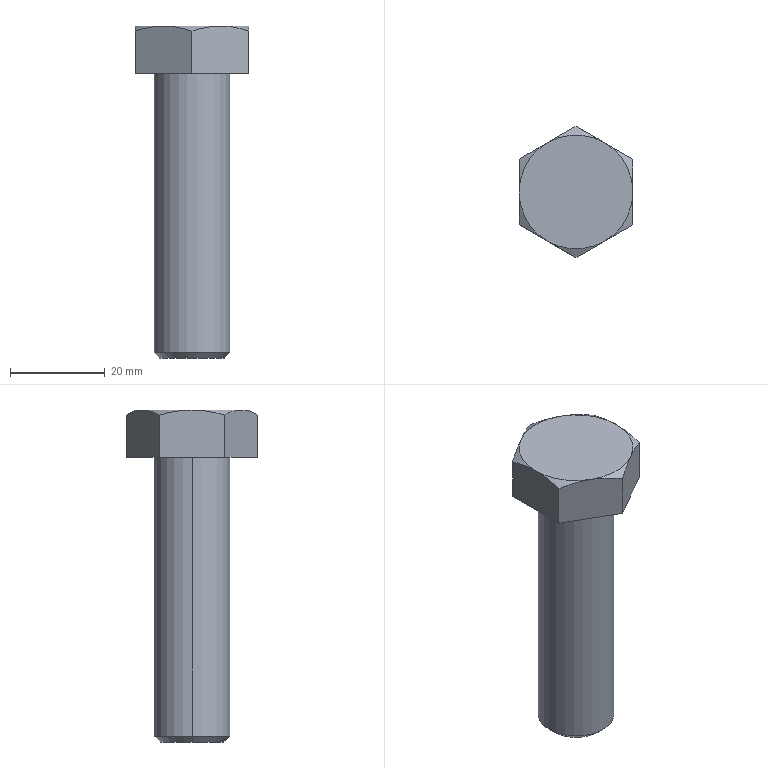Part | SolidWorks | features BaseBody 1 | 1 solid | 19 faces | box 24 x 27.713 x 70 mm | volume 17001 mm3 | plane 9 | cone 8 | cylinder 2 | commonest cylinder face diameters 16 x2
STEP:
#1=CARTESIAN_POINT('',(8.,0.,-38.773));
#2=VERTEX_POINT('',#1);
#3=CARTESIAN_POINT('',(-8.,0.,-38.773));
#4=VERTEX_POINT('',#3);
#5=CARTESIAN_POINT('',(0.,0.,-38.773));
#6=DIRECTION('',(0.,0.,1.));
#7=DIRECTION('',(1.,0.,0.));
#8=AXIS2_PLACEMENT_3D('',#5,#6,#7);
#9=CIRCLE('',#8,8.);
#10=EDGE_CURVE('',#2,#4,#9,.T.);
#11=ORIENTED_EDGE('',*,*,#10,.T.);
#12=CARTESIAN_POINT('',(-8.,0.,20.));
#13=VERTEX_POINT('',#12);
#14=CARTESIAN_POINT('',(-8.,0.,-100.));
#15=DIRECTION('',(0.,0.,1.));
#16=VECTOR('',#15,1000.);
#17=LINE('',#14,#16);
#18=EDGE_CURVE('',#4,#13,#17,.T.);
#19=ORIENTED_EDGE('',*,*,#18,.T.);
#20=CARTESIAN_POINT('',(8.,0.,20.));
#21=VERTEX_POINT('',#20);
#22=CARTESIAN_POINT('',(0.,0.,20.));
#23=DIRECTION('',(0.,0.,-1.));
#24=DIRECTION('',(1.,0.,0.));
#25=AXIS2_PLACEMENT_3D('',#22,#23,#24);
#26=CIRCLE('',#25,8.);
#27=EDGE_CURVE('',#13,#21,#26,.T.);
#28=ORIENTED_EDGE('',*,*,#27,.T.);
#29=CARTESIAN_POINT('',(8.,0.,-100.));
#30=DIRECTION('',(0.,0.,1.));
#31=VECTOR('',#30,1000.);
#32=LINE('',#29,#31);
#33=EDGE_CURVE('',#2,#21,#32,.T.);
#34=ORIENTED_EDGE('',*,*,#33,.F.);
#35=EDGE_LOOP('',(#11,#19,#28,#34));
#36=FACE_OUTER_BOUND('',#35,.T.);
#37=CARTESIAN_POINT('',(0.,0.,-100.));
#38=DIRECTION('',(0.,0.,1.));
#39=DIRECTION('',(1.,0.,0.));
#40=AXIS2_PLACEMENT_3D('',#37,#38,#39);
#41=CYLINDRICAL_SURFACE('',#40,8.);
#42=ADVANCED_FACE('',(#36),#41,.T.);
#43=CARTESIAN_POINT('',(6.773,0.,-40.));
#44=VERTEX_POINT('',#43);
#45=CARTESIAN_POINT('',(-6.773,0.,-40.));
#46=VERTEX_POINT('',#45);
#47=CARTESIAN_POINT('',(0.,0.,-40.));
#48=DIRECTION('',(0.,0.,1.));
#49=DIRECTION('',(1.,0.,0.));
#50=AXIS2_PLACEMENT_3D('',#47,#48,#49);
#51=CIRCLE('',#50,6.773);
#52=EDGE_CURVE('',#44,#46,#51,.T.);
#53=ORIENTED_EDGE('',*,*,#52,.T.);
#54=CARTESIAN_POINT('',(-8.,0.,-38.773));
#55=DIRECTION('',(-0.7071,0.,0.7071));
#56=VECTOR('',#55,1000.);
#57=LINE('',#54,#56);
#58=EDGE_CURVE('',#46,#4,#57,.T.);
#59=ORIENTED_EDGE('',*,*,#58,.T.);
#60=ORIENTED_EDGE('',*,*,#10,.F.);
#61=CARTESIAN_POINT('',(8.,0.,-38.773));
#62=DIRECTION('',(0.7071,0.,0.7071));
#63=VECTOR('',#62,1000.);
#64=LINE('',#61,#63);
#65=EDGE_CURVE('',#44,#2,#64,.T.);
#66=ORIENTED_EDGE('',*,*,#65,.F.);
#67=EDGE_LOOP('',(#53,#59,#60,#66));
#68=FACE_OUTER_BOUND('',#67,.T.);
#69=CARTESIAN_POINT('',(0.,0.,-38.773));
#70=DIRECTION('',(0.,0.,1.));
#71=DIRECTION('',(1.,0.,0.));
#72=AXIS2_PLACEMENT_3D('',#69,#70,#71);
#73=CONICAL_SURFACE('',#72,8.,0.7854);
#74=ADVANCED_FACE('',(#68),#73,.T.);
#75=ORIENTED_EDGE('',*,*,#18,.F.);
#76=CARTESIAN_POINT('',(0.,0.,-38.773));
#77=DIRECTION('',(0.,0.,1.));
#78=DIRECTION('',(1.,0.,0.));
#79=AXIS2_PLACEMENT_3D('',#76,#77,#78);
#80=CIRCLE('',#79,8.);
#81=EDGE_CURVE('',#4,#2,#80,.T.);
#82=ORIENTED_EDGE('',*,*,#81,.T.);
#83=ORIENTED_EDGE('',*,*,#33,.T.);
#84=CARTESIAN_POINT('',(0.,0.,20.));
#85=DIRECTION('',(0.,0.,-1.));
#86=DIRECTION('',(1.,0.,0.));
#87=AXIS2_PLACEMENT_3D('',#84,#85,#86);
#88=CIRCLE('',#87,8.);
#89=EDGE_CURVE('',#21,#13,#88,.T.);
#90=ORIENTED_EDGE('',*,*,#89,.T.);
#91=EDGE_LOOP('',(#75,#82,#83,#90));
#92=FACE_OUTER_BOUND('',#91,.T.);
#93=CARTESIAN_POINT('',(0.,0.,-100.));
#94=DIRECTION('',(0.,0.,1.));
#95=DIRECTION('',(1.,0.,0.));
#96=AXIS2_PLACEMENT_3D('',#93,#94,#95);
#97=CYLINDRICAL_SURFACE('',#96,8.);
#98=ADVANCED_FACE('',(#92),#97,.T.);
#99=ORIENTED_EDGE('',*,*,#89,.F.);
#100=ORIENTED_EDGE('',*,*,#27,.F.);
#101=EDGE_LOOP('',(#99,#100));
#102=FACE_BOUND('',#101,.T.);
#103=CARTESIAN_POINT('',(-12.,6.928,20.));
#104=VERTEX_POINT('',#103);
#105=CARTESIAN_POINT('',(-12.,-6.928,20.));
#106=VERTEX_POINT('',#105);
#107=CARTESIAN_POINT('',(-12.,0.,20.));
#108=DIRECTION('',(0.,-1.,0.));
#109=VECTOR('',#108,1000.);
#110=LINE('',#107,#109);
#111=EDGE_CURVE('',#104,#106,#110,.T.);
#112=ORIENTED_EDGE('',*,*,#111,.F.);
#113=CARTESIAN_POINT('',(0.,13.856,20.));
#114=VERTEX_POINT('',#113);
#115=CARTESIAN_POINT('',(0.,13.856,20.));
#116=DIRECTION('',(-0.866,-0.5,0.));
#117=VECTOR('',#116,1000.);
#118=LINE('',#115,#117);
#119=EDGE_CURVE('',#114,#104,#118,.T.);
#120=ORIENTED_EDGE('',*,*,#119,.F.);
#121=CARTESIAN_POINT('',(12.,6.928,20.));
#122=VERTEX_POINT('',#121);
#123=CARTESIAN_POINT('',(12.,6.928,20.));
#124=DIRECTION('',(-0.866,0.5,0.));
#125=VECTOR('',#124,1000.);
#126=LINE('',#123,#125);
#127=EDGE_CURVE('',#122,#114,#126,.T.);
#128=ORIENTED_EDGE('',*,*,#127,.F.);
#129=CARTESIAN_POINT('',(12.,-6.928,20.));
#130=VERTEX_POINT('',#129);
#131=CARTESIAN_POINT('',(12.,0.,20.));
#132=DIRECTION('',(0.,1.,0.));
#133=VECTOR('',#132,1000.);
#134=LINE('',#131,#133);
#135=EDGE_CURVE('',#130,#122,#134,.T.);
#136=ORIENTED_EDGE('',*,*,#135,.F.);
#137=CARTESIAN_POINT('',(0.,-13.856,20.));
#138=VERTEX_POINT('',#137);
#139=CARTESIAN_POINT('',(0.,-13.856,20.));
#140=DIRECTION('',(0.866,0.5,0.));
#141=VECTOR('',#140,1000.);
#142=LINE('',#139,#141);
#143=EDGE_CURVE('',#138,#130,#142,.T.);
#144=ORIENTED_EDGE('',*,*,#143,.F.);
#145=CARTESIAN_POINT('',(-12.,-6.928,20.));
#146=DIRECTION('',(0.866,-0.5,0.));
#147=VECTOR('',#146,1000.);
#148=LINE('',#145,#147);
#149=EDGE_CURVE('',#106,#138,#148,.T.);
#150=ORIENTED_EDGE('',*,*,#149,.F.);
#151=EDGE_LOOP('',(#112,#120,#128,#136,#144,#150));
#152=FACE_OUTER_BOUND('',#151,.T.);
#153=CARTESIAN_POINT('',(0.,0.,20.));
#154=DIRECTION('',(0.,0.,1.));
#155=DIRECTION('',(1.,0.,0.));
#156=AXIS2_PLACEMENT_3D('',#153,#154,#155);
#157=PLANE('',#156);
#158=ADVANCED_FACE('',(#102,#152),#157,.F.);
#159=ORIENTED_EDGE('',*,*,#58,.F.);
#160=CARTESIAN_POINT('',(0.,0.,-40.));
#161=DIRECTION('',(0.,0.,1.));
#162=DIRECTION('',(1.,0.,0.));
#163=AXIS2_PLACEMENT_3D('',#160,#161,#162);
#164=CIRCLE('',#163,6.773);
#165=EDGE_CURVE('',#46,#44,#164,.T.);
#166=ORIENTED_EDGE('',*,*,#165,.T.);
#167=ORIENTED_EDGE('',*,*,#65,.T.);
#168=ORIENTED_EDGE('',*,*,#81,.F.);
#169=EDGE_LOOP('',(#159,#166,#167,#168));
#170=FACE_OUTER_BOUND('',#169,.T.);
#171=CARTESIAN_POINT('',(0.,0.,-38.773));
#172=DIRECTION('',(0.,0.,1.));
#173=DIRECTION('',(1.,0.,0.));
#174=AXIS2_PLACEMENT_3D('',#171,#172,#173);
#175=CONICAL_SURFACE('',#174,8.,0.7854);
#176=ADVANCED_FACE('',(#170),#175,.T.);
#177=CARTESIAN_POINT('',(-6.,-10.392,30.));
#178=VERTEX_POINT('',#177);
#179=CARTESIAN_POINT('',(0.,-13.856,28.928));
#180=VERTEX_POINT('',#179);
#181=CARTESIAN_POINT('',(-6.,-10.392,30.));
#182=CARTESIAN_POINT('',(-4.976,-10.983,30.));
#183=CARTESIAN_POINT('',(-3.966,-11.567,29.898));
#184=CARTESIAN_POINT('',(-1.968,-12.72,29.524));
#185=CARTESIAN_POINT('',(-0.9802,-13.291,29.255));
#186=CARTESIAN_POINT('',(0.,-13.856,28.928));
#187=B_SPLINE_CURVE_WITH_KNOTS('',3,(#181,#182,#183,#184,#185,#186),.UNSPECIFIED.,.F.,.F.,(4,2,4),(0.,0.003505,0.007011),.UNSPECIFIED.);
#188=EDGE_CURVE('',#178,#180,#187,.T.);
#189=ORIENTED_EDGE('',*,*,#188,.F.);
#190=CARTESIAN_POINT('',(-12.,-6.928,28.928));
#191=VERTEX_POINT('',#190);
#192=CARTESIAN_POINT('',(-12.,-6.928,28.928));
#193=CARTESIAN_POINT('',(-11.02,-7.494,29.255));
#194=CARTESIAN_POINT('',(-10.032,-8.064,29.524));
#195=CARTESIAN_POINT('',(-8.034,-9.218,29.898));
#196=CARTESIAN_POINT('',(-7.024,-9.801,30.));
#197=CARTESIAN_POINT('',(-6.,-10.392,30.));
#198=B_SPLINE_CURVE_WITH_KNOTS('',3,(#192,#193,#194,#195,#196,#197),.UNSPECIFIED.,.F.,.F.,(4,2,4),(0.,0.003505,0.007011),.UNSPECIFIED.);
#199=EDGE_CURVE('',#191,#178,#198,.T.);
#200=ORIENTED_EDGE('',*,*,#199,.F.);
#201=CARTESIAN_POINT('',(-12.,-6.928,30.));
#202=DIRECTION('',(0.,0.,1.));
#203=VECTOR('',#202,1000.);
#204=LINE('',#201,#203);
#205=EDGE_CURVE('',#106,#191,#204,.T.);
#206=ORIENTED_EDGE('',*,*,#205,.F.);
#207=ORIENTED_EDGE('',*,*,#149,.T.);
#208=CARTESIAN_POINT('',(0.,-13.856,30.));
#209=DIRECTION('',(0.,0.,-1.));
#210=VECTOR('',#209,1000.);
#211=LINE('',#208,#210);
#212=EDGE_CURVE('',#180,#138,#211,.T.);
#213=ORIENTED_EDGE('',*,*,#212,.F.);
#214=EDGE_LOOP('',(#189,#200,#206,#207,#213));
#215=FACE_OUTER_BOUND('',#214,.T.);
#216=CARTESIAN_POINT('',(-12.,-6.928,30.));
#217=DIRECTION('',(0.5,0.866,0.));
#218=DIRECTION('',(-0.866,0.5,0.));
#219=AXIS2_PLACEMENT_3D('',#216,#217,#218);
#220=PLANE('',#219);
#221=ADVANCED_FACE('',(#215),#220,.F.);
#222=CARTESIAN_POINT('',(-12.,0.,30.));
#223=VERTEX_POINT('',#222);
#224=CARTESIAN_POINT('',(-12.,0.,30.));
#225=CARTESIAN_POINT('',(-12.,-1.182,30.));
#226=CARTESIAN_POINT('',(-12.,-2.349,29.898));
#227=CARTESIAN_POINT('',(-12.,-4.656,29.524));
#228=CARTESIAN_POINT('',(-12.,-5.796,29.255));
#229=CARTESIAN_POINT('',(-12.,-6.928,28.928));
#230=B_SPLINE_CURVE_WITH_KNOTS('',3,(#224,#225,#226,#227,#228,#229),.UNSPECIFIED.,.F.,.F.,(4,2,4),(0.,0.003505,0.007011),.UNSPECIFIED.);
#231=EDGE_CURVE('',#223,#191,#230,.T.);
#232=ORIENTED_EDGE('',*,*,#231,.F.);
#233=CARTESIAN_POINT('',(-12.,6.928,28.928));
#234=VERTEX_POINT('',#233);
#235=CARTESIAN_POINT('',(-12.,6.928,28.928));
#236=CARTESIAN_POINT('',(-12.,5.796,29.255));
#237=CARTESIAN_POINT('',(-12.,4.656,29.524));
#238=CARTESIAN_POINT('',(-12.,2.349,29.898));
#239=CARTESIAN_POINT('',(-12.,1.182,30.));
#240=CARTESIAN_POINT('',(-12.,0.,30.));
#241=B_SPLINE_CURVE_WITH_KNOTS('',3,(#235,#236,#237,#238,#239,#240),.UNSPECIFIED.,.F.,.F.,(4,2,4),(0.,0.003505,0.007011),.UNSPECIFIED.);
#242=EDGE_CURVE('',#234,#223,#241,.T.);
#243=ORIENTED_EDGE('',*,*,#242,.F.);
#244=CARTESIAN_POINT('',(-12.,6.928,30.));
#245=DIRECTION('',(0.,0.,1.));
#246=VECTOR('',#245,1000.);
#247=LINE('',#244,#246);
#248=EDGE_CURVE('',#104,#234,#247,.T.);
#249=ORIENTED_EDGE('',*,*,#248,.F.);
#250=ORIENTED_EDGE('',*,*,#111,.T.);
#251=ORIENTED_EDGE('',*,*,#205,.T.);
#252=EDGE_LOOP('',(#232,#243,#249,#250,#251));
#253=FACE_OUTER_BOUND('',#252,.T.);
#254=CARTESIAN_POINT('',(-12.,6.928,30.));
#255=DIRECTION('',(1.,0.,0.));
#256=DIRECTION('',(0.,0.,-1.));
#257=AXIS2_PLACEMENT_3D('',#254,#255,#256);
#258=PLANE('',#257);
#259=ADVANCED_FACE('',(#253),#258,.F.);
#260=CARTESIAN_POINT('',(-6.,10.392,30.));
#261=VERTEX_POINT('',#260);
#262=CARTESIAN_POINT('',(-6.,10.392,30.));
#263=CARTESIAN_POINT('',(-7.024,9.801,30.));
#264=CARTESIAN_POINT('',(-8.034,9.218,29.898));
#265=CARTESIAN_POINT('',(-10.032,8.064,29.524));
#266=CARTESIAN_POINT('',(-11.02,7.494,29.255));
#267=CARTESIAN_POINT('',(-12.,6.928,28.928));
#268=B_SPLINE_CURVE_WITH_KNOTS('',3,(#262,#263,#264,#265,#266,#267),.UNSPECIFIED.,.F.,.F.,(4,2,4),(0.,0.003505,0.007011),.UNSPECIFIED.);
#269=EDGE_CURVE('',#261,#234,#268,.T.);
#270=ORIENTED_EDGE('',*,*,#269,.F.);
#271=CARTESIAN_POINT('',(0.,13.856,28.928));
#272=VERTEX_POINT('',#271);
#273=CARTESIAN_POINT('',(0.,13.856,28.928));
#274=CARTESIAN_POINT('',(-0.9802,13.291,29.255));
#275=CARTESIAN_POINT('',(-1.968,12.72,29.524));
#276=CARTESIAN_POINT('',(-3.966,11.567,29.898));
#277=CARTESIAN_POINT('',(-4.976,10.983,30.));
#278=CARTESIAN_POINT('',(-6.,10.392,30.));
#279=B_SPLINE_CURVE_WITH_KNOTS('',3,(#273,#274,#275,#276,#277,#278),.UNSPECIFIED.,.F.,.F.,(4,2,4),(0.,0.003505,0.007011),.UNSPECIFIED.);
#280=EDGE_CURVE('',#272,#261,#279,.T.);
#281=ORIENTED_EDGE('',*,*,#280,.F.);
#282=CARTESIAN_POINT('',(0.,13.856,30.));
#283=DIRECTION('',(0.,0.,1.));
#284=VECTOR('',#283,1000.);
#285=LINE('',#282,#284);
#286=EDGE_CURVE('',#114,#272,#285,.T.);
#287=ORIENTED_EDGE('',*,*,#286,.F.);
#288=ORIENTED_EDGE('',*,*,#119,.T.);
#289=ORIENTED_EDGE('',*,*,#248,.T.);
#290=EDGE_LOOP('',(#270,#281,#287,#288,#289));
#291=FACE_OUTER_BOUND('',#290,.T.);
#292=CARTESIAN_POINT('',(0.,13.856,30.));
#293=DIRECTION('',(0.5,-0.866,0.));
#294=DIRECTION('',(0.866,0.5,0.));
#295=AXIS2_PLACEMENT_3D('',#292,#293,#294);
#296=PLANE('',#295);
#297=ADVANCED_FACE('',(#291),#296,.F.);
#298=CARTESIAN_POINT('',(6.,10.392,30.));
#299=VERTEX_POINT('',#298);
#300=CARTESIAN_POINT('',(6.,10.392,30.));
#301=CARTESIAN_POINT('',(4.976,10.983,30.));
#302=CARTESIAN_POINT('',(3.966,11.567,29.898));
#303=CARTESIAN_POINT('',(1.968,12.72,29.524));
#304=CARTESIAN_POINT('',(0.9802,13.291,29.255));
#305=CARTESIAN_POINT('',(0.,13.856,28.928));
#306=B_SPLINE_CURVE_WITH_KNOTS('',3,(#300,#301,#302,#303,#304,#305),.UNSPECIFIED.,.F.,.F.,(4,2,4),(0.,0.003505,0.007011),.UNSPECIFIED.);
#307=EDGE_CURVE('',#299,#272,#306,.T.);
#308=ORIENTED_EDGE('',*,*,#307,.F.);
#309=CARTESIAN_POINT('',(12.,6.928,28.928));
#310=VERTEX_POINT('',#309);
#311=CARTESIAN_POINT('',(12.,6.928,28.928));
#312=CARTESIAN_POINT('',(11.02,7.494,29.255));
#313=CARTESIAN_POINT('',(10.032,8.064,29.524));
#314=CARTESIAN_POINT('',(8.034,9.218,29.898));
#315=CARTESIAN_POINT('',(7.024,9.801,30.));
#316=CARTESIAN_POINT('',(6.,10.392,30.));
#317=B_SPLINE_CURVE_WITH_KNOTS('',3,(#311,#312,#313,#314,#315,#316),.UNSPECIFIED.,.F.,.F.,(4,2,4),(0.,0.003505,0.007011),.UNSPECIFIED.);
#318=EDGE_CURVE('',#310,#299,#317,.T.);
#319=ORIENTED_EDGE('',*,*,#318,.F.);
#320=CARTESIAN_POINT('',(12.,6.928,30.));
#321=DIRECTION('',(0.,0.,1.));
#322=VECTOR('',#321,1000.);
#323=LINE('',#320,#322);
#324=EDGE_CURVE('',#122,#310,#323,.T.);
#325=ORIENTED_EDGE('',*,*,#324,.F.);
#326=ORIENTED_EDGE('',*,*,#127,.T.);
#327=ORIENTED_EDGE('',*,*,#286,.T.);
#328=EDGE_LOOP('',(#308,#319,#325,#326,#327));
#329=FACE_OUTER_BOUND('',#328,.T.);
#330=CARTESIAN_POINT('',(12.,6.928,30.));
#331=DIRECTION('',(-0.5,-0.866,0.));
#332=DIRECTION('',(0.866,-0.5,0.));
#333=AXIS2_PLACEMENT_3D('',#330,#331,#332);
#334=PLANE('',#333);
#335=ADVANCED_FACE('',(#329),#334,.F.);
#336=CARTESIAN_POINT('',(12.,0.,30.));
#337=VERTEX_POINT('',#336);
#338=CARTESIAN_POINT('',(12.,0.,30.));
#339=CARTESIAN_POINT('',(12.,1.182,30.));
#340=CARTESIAN_POINT('',(12.,2.349,29.898));
#341=CARTESIAN_POINT('',(12.,4.656,29.524));
#342=CARTESIAN_POINT('',(12.,5.796,29.255));
#343=CARTESIAN_POINT('',(12.,6.928,28.928));
#344=B_SPLINE_CURVE_WITH_KNOTS('',3,(#338,#339,#340,#341,#342,#343),.UNSPECIFIED.,.F.,.F.,(4,2,4),(0.,0.003505,0.007011),.UNSPECIFIED.);
#345=EDGE_CURVE('',#337,#310,#344,.T.);
#346=ORIENTED_EDGE('',*,*,#345,.F.);
#347=CARTESIAN_POINT('',(12.,-6.928,28.928));
#348=VERTEX_POINT('',#347);
#349=CARTESIAN_POINT('',(12.,-6.928,28.928));
#350=CARTESIAN_POINT('',(12.,-5.796,29.255));
#351=CARTESIAN_POINT('',(12.,-4.656,29.524));
#352=CARTESIAN_POINT('',(12.,-2.349,29.898));
#353=CARTESIAN_POINT('',(12.,-1.182,30.));
#354=CARTESIAN_POINT('',(12.,0.,30.));
#355=B_SPLINE_CURVE_WITH_KNOTS('',3,(#349,#350,#351,#352,#353,#354),.UNSPECIFIED.,.F.,.F.,(4,2,4),(0.,0.003505,0.007011),.UNSPECIFIED.);
#356=EDGE_CURVE('',#348,#337,#355,.T.);
#357=ORIENTED_EDGE('',*,*,#356,.F.);
#358=CARTESIAN_POINT('',(12.,-6.928,30.));
#359=DIRECTION('',(0.,0.,1.));
#360=VECTOR('',#359,1000.);
#361=LINE('',#358,#360);
#362=EDGE_CURVE('',#130,#348,#361,.T.);
#363=ORIENTED_EDGE('',*,*,#362,.F.);
#364=ORIENTED_EDGE('',*,*,#135,.T.);
#365=ORIENTED_EDGE('',*,*,#324,.T.);
#366=EDGE_LOOP('',(#346,#357,#363,#364,#365));
#367=FACE_OUTER_BOUND('',#366,.T.);
#368=CARTESIAN_POINT('',(12.,-6.928,30.));
#369=DIRECTION('',(-1.,0.,0.));
#370=DIRECTION('',(0.,0.,1.));
#371=AXIS2_PLACEMENT_3D('',#368,#369,#370);
#372=PLANE('',#371);
#373=ADVANCED_FACE('',(#367),#372,.F.);
#374=CARTESIAN_POINT('',(6.,-10.392,30.));
#375=VERTEX_POINT('',#374);
#376=CARTESIAN_POINT('',(6.,-10.392,30.));
#377=CARTESIAN_POINT('',(7.024,-9.801,30.));
#378=CARTESIAN_POINT('',(8.034,-9.218,29.898));
#379=CARTESIAN_POINT('',(10.032,-8.064,29.524));
#380=CARTESIAN_POINT('',(11.02,-7.494,29.255));
#381=CARTESIAN_POINT('',(12.,-6.928,28.928));
#382=B_SPLINE_CURVE_WITH_KNOTS('',3,(#376,#377,#378,#379,#380,#381),.UNSPECIFIED.,.F.,.F.,(4,2,4),(0.,0.003505,0.007011),.UNSPECIFIED.);
#383=EDGE_CURVE('',#375,#348,#382,.T.);
#384=ORIENTED_EDGE('',*,*,#383,.F.);
#385=CARTESIAN_POINT('',(0.,-13.856,28.928));
#386=CARTESIAN_POINT('',(0.9802,-13.291,29.255));
#387=CARTESIAN_POINT('',(1.968,-12.72,29.524));
#388=CARTESIAN_POINT('',(3.966,-11.567,29.898));
#389=CARTESIAN_POINT('',(4.976,-10.983,30.));
#390=CARTESIAN_POINT('',(6.,-10.392,30.));
#391=B_SPLINE_CURVE_WITH_KNOTS('',3,(#385,#386,#387,#388,#389,#390),.UNSPECIFIED.,.F.,.F.,(4,2,4),(0.,0.003505,0.007011),.UNSPECIFIED.);
#392=EDGE_CURVE('',#180,#375,#391,.T.);
#393=ORIENTED_EDGE('',*,*,#392,.F.);
#394=ORIENTED_EDGE('',*,*,#212,.T.);
#395=ORIENTED_EDGE('',*,*,#143,.T.);
#396=ORIENTED_EDGE('',*,*,#362,.T.);
#397=EDGE_LOOP('',(#384,#393,#394,#395,#396));
#398=FACE_OUTER_BOUND('',#397,.T.);
#399=CARTESIAN_POINT('',(0.,-13.856,30.));
#400=DIRECTION('',(-0.5,0.866,0.));
#401=DIRECTION('',(-0.866,-0.5,0.));
#402=AXIS2_PLACEMENT_3D('',#399,#400,#401);
#403=PLANE('',#402);
#404=ADVANCED_FACE('',(#398),#403,.F.);
#405=ORIENTED_EDGE('',*,*,#52,.F.);
#406=ORIENTED_EDGE('',*,*,#165,.F.);
#407=EDGE_LOOP('',(#405,#406));
#408=FACE_OUTER_BOUND('',#407,.T.);
#409=CARTESIAN_POINT('',(0.,6.773,-40.));
#410=DIRECTION('',(0.,0.,1.));
#411=DIRECTION('',(1.,0.,0.));
#412=AXIS2_PLACEMENT_3D('',#409,#410,#411);
#413=PLANE('',#412);
#414=ADVANCED_FACE('',(#408),#413,.F.);
#415=ORIENTED_EDGE('',*,*,#188,.T.);
#416=ORIENTED_EDGE('',*,*,#392,.T.);
#417=CARTESIAN_POINT('',(0.,0.,30.));
#418=DIRECTION('',(0.,0.,-1.));
#419=DIRECTION('',(-1.,0.,0.));
#420=AXIS2_PLACEMENT_3D('',#417,#418,#419);
#421=CIRCLE('',#420,12.);
#422=EDGE_CURVE('',#375,#178,#421,.T.);
#423=ORIENTED_EDGE('',*,*,#422,.T.);
#424=EDGE_LOOP('',(#415,#416,#423));
#425=FACE_OUTER_BOUND('',#424,.T.);
#426=CARTESIAN_POINT('',(0.,0.,28.922));
#427=DIRECTION('',(0.,0.,-1.));
#428=DIRECTION('',(-1.,0.,0.));
#429=AXIS2_PLACEMENT_3D('',#426,#427,#428);
#430=CONICAL_SURFACE('',#429,13.868,1.047);
#431=ADVANCED_FACE('',(#425),#430,.T.);
#432=ORIENTED_EDGE('',*,*,#231,.T.);
#433=ORIENTED_EDGE('',*,*,#199,.T.);
#434=CARTESIAN_POINT('',(0.,0.,30.));
#435=DIRECTION('',(0.,0.,-1.));
#436=DIRECTION('',(-1.,0.,0.));
#437=AXIS2_PLACEMENT_3D('',#434,#435,#436);
#438=CIRCLE('',#437,12.);
#439=EDGE_CURVE('',#178,#223,#438,.T.);
#440=ORIENTED_EDGE('',*,*,#439,.T.);
#441=EDGE_LOOP('',(#432,#433,#440));
#442=FACE_OUTER_BOUND('',#441,.T.);
#443=CARTESIAN_POINT('',(0.,0.,28.922));
#444=DIRECTION('',(0.,0.,-1.));
#445=DIRECTION('',(-1.,0.,0.));
#446=AXIS2_PLACEMENT_3D('',#443,#444,#445);
#447=CONICAL_SURFACE('',#446,13.868,1.047);
#448=ADVANCED_FACE('',(#442),#447,.T.);
#449=CARTESIAN_POINT('',(0.,0.,30.));
#450=DIRECTION('',(0.,0.,-1.));
#451=DIRECTION('',(-1.,0.,0.));
#452=AXIS2_PLACEMENT_3D('',#449,#450,#451);
#453=CIRCLE('',#452,12.);
#454=EDGE_CURVE('',#223,#261,#453,.T.);
#455=ORIENTED_EDGE('',*,*,#454,.T.);
#456=ORIENTED_EDGE('',*,*,#269,.T.);
#457=ORIENTED_EDGE('',*,*,#242,.T.);
#458=EDGE_LOOP('',(#455,#456,#457));
#459=FACE_OUTER_BOUND('',#458,.T.);
#460=CARTESIAN_POINT('',(0.,0.,28.922));
#461=DIRECTION('',(0.,0.,-1.));
#462=DIRECTION('',(-1.,0.,0.));
#463=AXIS2_PLACEMENT_3D('',#460,#461,#462);
#464=CONICAL_SURFACE('',#463,13.868,1.047);
#465=ADVANCED_FACE('',(#459),#464,.T.);
#466=ORIENTED_EDGE('',*,*,#280,.T.);
#467=CARTESIAN_POINT('',(0.,0.,30.));
#468=DIRECTION('',(0.,0.,-1.));
#469=DIRECTION('',(-1.,0.,0.));
#470=AXIS2_PLACEMENT_3D('',#467,#468,#469);
#471=CIRCLE('',#470,12.);
#472=EDGE_CURVE('',#261,#299,#471,.T.);
#473=ORIENTED_EDGE('',*,*,#472,.T.);
#474=ORIENTED_EDGE('',*,*,#307,.T.);
#475=EDGE_LOOP('',(#466,#473,#474));
#476=FACE_OUTER_BOUND('',#475,.T.);
#477=CARTESIAN_POINT('',(0.,0.,28.922));
#478=DIRECTION('',(0.,0.,-1.));
#479=DIRECTION('',(-1.,0.,0.));
#480=AXIS2_PLACEMENT_3D('',#477,#478,#479);
#481=CONICAL_SURFACE('',#480,13.868,1.047);
#482=ADVANCED_FACE('',(#476),#481,.T.);
#483=CARTESIAN_POINT('',(0.,0.,30.));
#484=DIRECTION('',(0.,0.,-1.));
#485=DIRECTION('',(-1.,0.,0.));
#486=AXIS2_PLACEMENT_3D('',#483,#484,#485);
#487=CIRCLE('',#486,12.);
#488=EDGE_CURVE('',#299,#337,#487,.T.);
#489=ORIENTED_EDGE('',*,*,#488,.T.);
#490=ORIENTED_EDGE('',*,*,#345,.T.);
#491=ORIENTED_EDGE('',*,*,#318,.T.);
#492=EDGE_LOOP('',(#489,#490,#491));
#493=FACE_OUTER_BOUND('',#492,.T.);
#494=CARTESIAN_POINT('',(0.,0.,28.922));
#495=DIRECTION('',(0.,0.,-1.));
#496=DIRECTION('',(-1.,0.,0.));
#497=AXIS2_PLACEMENT_3D('',#494,#495,#496);
#498=CONICAL_SURFACE('',#497,13.868,1.047);
#499=ADVANCED_FACE('',(#493),#498,.T.);
#500=ORIENTED_EDGE('',*,*,#383,.T.);
#501=ORIENTED_EDGE('',*,*,#356,.T.);
#502=CARTESIAN_POINT('',(0.,0.,30.));
#503=DIRECTION('',(0.,0.,-1.));
#504=DIRECTION('',(-1.,0.,0.));
#505=AXIS2_PLACEMENT_3D('',#502,#503,#504);
#506=CIRCLE('',#505,12.);
#507=EDGE_CURVE('',#337,#375,#506,.T.);
#508=ORIENTED_EDGE('',*,*,#507,.T.);
#509=EDGE_LOOP('',(#500,#501,#508));
#510=FACE_OUTER_BOUND('',#509,.T.);
#511=CARTESIAN_POINT('',(0.,0.,28.922));
#512=DIRECTION('',(0.,0.,-1.));
#513=DIRECTION('',(-1.,0.,0.));
#514=AXIS2_PLACEMENT_3D('',#511,#512,#513);
#515=CONICAL_SURFACE('',#514,13.868,1.047);
#516=ADVANCED_FACE('',(#510),#515,.T.);
#517=ORIENTED_EDGE('',*,*,#454,.F.);
#518=ORIENTED_EDGE('',*,*,#439,.F.);
#519=ORIENTED_EDGE('',*,*,#422,.F.);
#520=ORIENTED_EDGE('',*,*,#507,.F.);
#521=ORIENTED_EDGE('',*,*,#488,.F.);
#522=ORIENTED_EDGE('',*,*,#472,.F.);
#523=EDGE_LOOP('',(#517,#518,#519,#520,#521,#522));
#524=FACE_OUTER_BOUND('',#523,.T.);
#525=CARTESIAN_POINT('',(0.,0.,30.));
#526=DIRECTION('',(0.,0.,1.));
#527=DIRECTION('',(1.,0.,0.));
#528=AXIS2_PLACEMENT_3D('',#525,#526,#527);
#529=PLANE('',#528);
#530=ADVANCED_FACE('',(#524),#529,.T.);
#531=CLOSED_SHELL('',(#42,#74,#98,#158,#176,#221,#259,#297,#335,#373,#404,#414,#431,#448,#465,#482,#499,#516,#530));
#532=MANIFOLD_SOLID_BREP('',#531);
#533=CARTESIAN_POINT('',(0.,0.,0.));
#534=DIRECTION('',(0.,0.,1.));
#535=DIRECTION('',(1.,0.,0.));
#536=AXIS2_PLACEMENT_3D('',#533,#534,#535);
#537=(LENGTH_UNIT()NAMED_UNIT(*)SI_UNIT(.MILLI.,.METRE.));
#538=UNCERTAINTY_MEASURE_WITH_UNIT(LENGTH_MEASURE(0.00001),#537,'','');
#539=(NAMED_UNIT(*)PLANE_ANGLE_UNIT()SI_UNIT($,.RADIAN.));
#540=(NAMED_UNIT(*)SI_UNIT($,.STERADIAN.)SOLID_ANGLE_UNIT());
#541=(GEOMETRIC_REPRESENTATION_CONTEXT(3)GLOBAL_UNCERTAINTY_ASSIGNED_CONTEXT((#538))GLOBAL_UNIT_ASSIGNED_CONTEXT((#537,#539,#540))REPRESENTATION_CONTEXT('',''));
#542=ADVANCED_BREP_SHAPE_REPRESENTATION('',(#532,#536),#541);